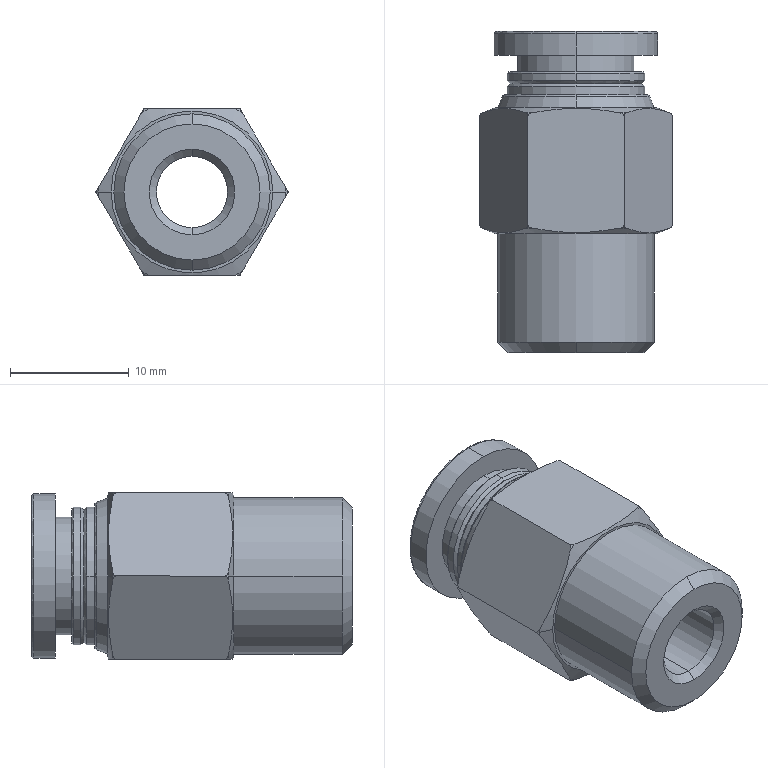Part | SolidWorks | features BaseBody 1 | 1 solid | 62 faces | box 16.166 x 27 x 14 mm | volume 2706 mm3 | spline 18 | cone 16 | cylinder 14 | plane 14 | commonest cylinder face diameters 11.6 x4 6 x2 8 x2 9.9 x2 13.157 x2 13.8 x2